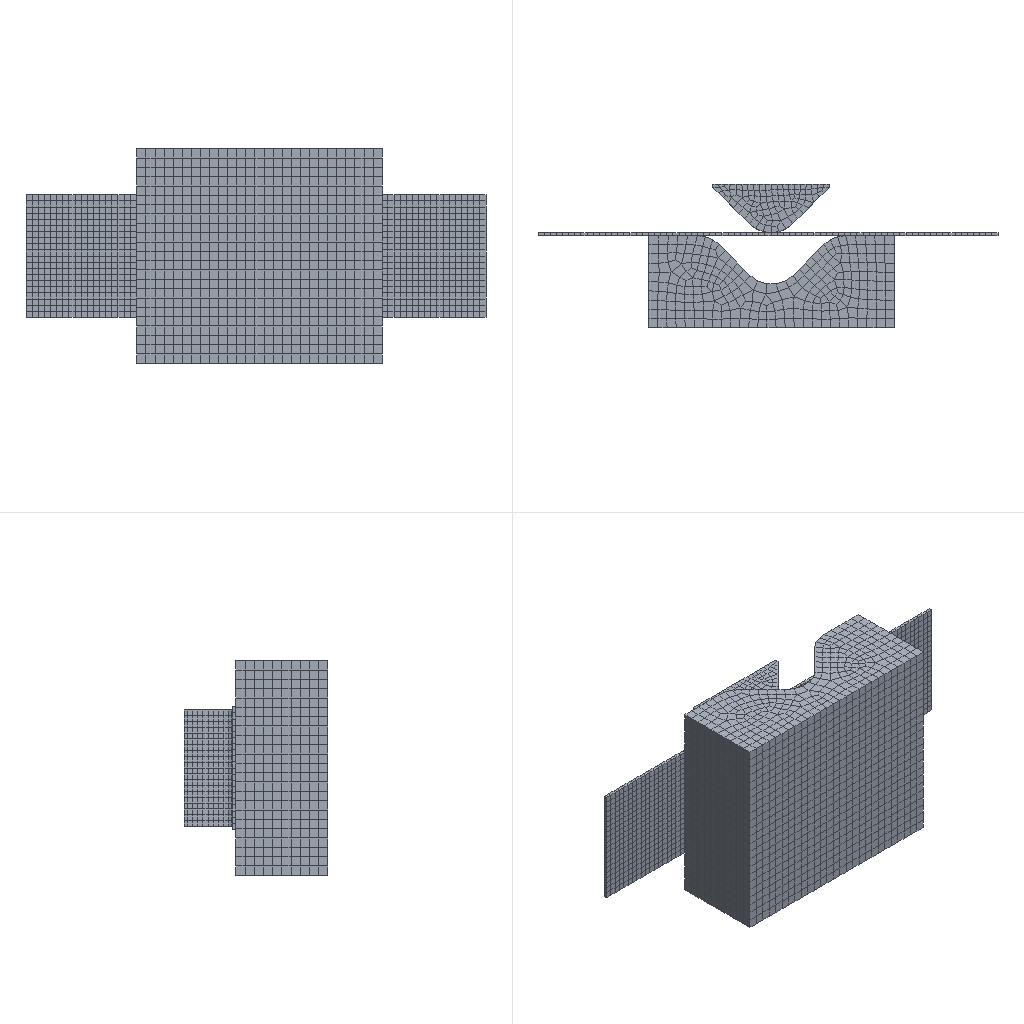Simulation study | abaqus
Set-up summary:
category,name,step,type,value,unit,region
solver,abaqus
solver,version,,,Abaqus/Standard 2020
units,not stated in the deck,,not stated
analysis,deck,,coupled temperature-displacement,coupled temperature-displacement
load_step,Step-1,Step-1,coupled temperature-displacement
load_step,Step-2,Step-2,coupled temperature-displacement
load_step,requested,,,2
mesh,nodes,,,12858
mesh,elements,,,9388
element_type,Q3D8R,,solid,9388
load,load commands in deck,,count,6
bc,support commands in deck,,count,21
material,BAN,,in results
material,MUJU,,in results
check,setup vs results,,match,"per instance, exact: element labels, types and connectivity; labels of the nodes the elements use; coordinates of those nodes at SINGLE_PRECISION in 3 of 3 instance(s)"
Abaqus input file, long lists of numbers shortened:
*Heading
** Job name: Job-1 Model name: Model-1
** Generated by: Abaqus/CAE 2020
*Preprint, echo=NO, model=NO, history=NO, contact=NO
**
** PARTS
**
*Part, name=work-1
*Node
      1,   160.87,   83.81,   69.627
      2,   158.87,   83.81,   69.627
** (3190 more lines like these left out)
*Element, type=Q3D8R
   1,  153,  154,  230,  229,    1,    2,   78,   77
   2,  154,  155,  231,  230,    2,    3,   79,   78
** (1498 more lines like these left out)
*Nset, nset=Set-1, generate
    1,  3192,     1
*Elset, elset=Set-1, generate
    1,  1500,     1
** Section: ban
*Solid Section, elset=Set-1, material=ban
,
*End Part
**
*Part, name=work-2
*Node
      1,   94.45,   95.668,    70.785
      2,   106.379,   107.597,    70.785
** (2560 more lines like these left out)
*Element, type=Q3D8R
   1,  117,  116,   86,  115,  239,  238,  208,  237
   2,   58,   69,   48,   45,  180,  191,  170,  167
** (1998 more lines like these left out)
*Nset, nset=Set-1, generate
    1,  2562,     1
*Elset, elset=Set-1, generate
    1,  2000,     1
** Section: muju
*Solid Section, elset=Set-1, material=muju
,
*End Part
**
*Part, name=work-3
*Node
      1,   111.165,   83.81,   124.661
      2,   127.022,   83.81,   124.661
** (7102 more lines like these left out)
*Element, type=Q3D8R
   1,  114,  185,   20,   21,  410,  481,  316,  317
   2,   85,   25,    5,   81,  381,  321,  301,  377
** (5886 more lines like these left out)
*Nset, nset=Set-1, generate
    1,  7104,     1
*Elset, elset=Set-1, generate
    1,  5888,     1
** Section: muju
*Solid Section, elset=Set-1, material=muju
,
*End Part
**
**
** ASSEMBLY
**
*Assembly, name=Assembly
**
*Instance, name=work-1-1, part=work-1
  -47.022,   -53.81,  -124.661
*End Instance
**
*Instance, name=work-2-1, part=work-2
  -47.531,   -61.739,   -124.819
*End Instance
**
*Instance, name=work-3-1, part=work-3
  -47.022,   -53.81,  -124.661
*End Instance
**
*Nset, nset=Set-1, instance=work-3-1
   16,   17,   44,   45,   46,   47,   48,   49,   50,   51,   52,   53,   54,   55,   56,   57
   58,   59,   60,   61,   62,   63,   64,   65,   66,   67,   68,   69,  312,  313,  340,  341
** (40 more lines like these left out)
*Elset, elset=Set-1, instance=work-3-1
    4,    5,    7,   20,   22,   34,   35,   36,   37,   39,   42,   43,   47,   49,   52,   57
   58,   61,   62,   77,   80,   82,   86,   88,   90,   98,  101,  260,  261,  263,  276,  278
** (37 more lines like these left out)
*Nset, nset=Set-2, instance=work-1-1, generate
    1,  3117,    76
*Elset, elset=Set-2, instance=work-1-1, generate
    1,  1426,    75
*Nset, nset=Set-3, instance=work-2-1
   10,   11,   24,   25,   26,   27,   28,   29,   30,   31,   32,   33,   34,   35,   36,   37
   38,   39,   40,   41,   42,  132,  133,  146,  147,  148,  149,  150,  151,  152,  153,  154
** (26 more lines like these left out)
*Elset, elset=Set-3, instance=work-2-1
    3,    5,    6,    7,   11,   15,   17,   18,   22,   24,   25,   26,   28,   32,   36,   41
   42,   47,   51,   78,  103,  105,  106,  107,  111,  115,  117,  118,  122,  124,  125,  126
** (23 more lines like these left out)
*Nset, nset=Set-4, instance=work-1-1, generate
    1,  3192,     1
*Nset, nset=Set-4, instance=work-2-1, generate
    1,  2562,     1
*Nset, nset=Set-4, instance=work-3-1, generate
    1,  7104,     1
*Elset, elset=Set-4, instance=work-1-1, generate
    1,  1500,     1
*Elset, elset=Set-4, instance=work-2-1, generate
    1,  2000,     1
*Elset, elset=Set-4, instance=work-3-1, generate
    1,  5888,     1
*Nset, nset=Set-5, instance=work-1-1
    1,   76,   77,  152,  153,  228,  229,  304,  305,  380,  381,  456,  457,  532,  533,  608
  609,  684,  685,  760,  761,  836,  837,  912,  913,  988,  989, 1064, 1065, 1140, 1141, 1216
** (4 more lines like these left out)
*Elset, elset=Set-5, instance=work-1-1
    1,   75,   76,  150,  151,  225,  226,  300,  301,  375,  376,  450,  451,  525,  526,  600
  601,  675,  676,  750,  751,  825,  826,  900,  901,  975,  976, 1050, 1051, 1125, 1126, 1200
** (1 more lines like these left out)
*Nset, nset=Set-6, instance=work-1-1
    1,   76,   77,  152,  153,  228,  229,  304,  305,  380,  381,  456,  457,  532,  533,  608
  609,  684,  685,  760,  761,  836,  837,  912,  913,  988,  989, 1064, 1065, 1140, 1141, 1216
** (4 more lines like these left out)
*Elset, elset=Set-6, instance=work-1-1
    1,   75,   76,  150,  151,  225,  226,  300,  301,  375,  376,  450,  451,  525,  526,  600
  601,  675,  676,  750,  751,  825,  826,  900,  901,  975,  976, 1050, 1051, 1125, 1126, 1200
** (1 more lines like these left out)
*Elset, elset=_Surf-1_S4, internal, instance=work-1-1, generate
   75,  1500,    75
*Surface, type=ELEMENT, name=Surf-1
_Surf-1_S4, S4
*Elset, elset=_Surf-6_S1, internal, instance=work-1-1, generate
 1426,  1500,     1
*Elset, elset=_Surf-6_S6, internal, instance=work-1-1, generate
    1,  1426,    75
*Elset, elset=_Surf-6_S2, internal, instance=work-1-1, generate
  1,  75,   1
*Elset, elset=_Surf-6_S4, internal, instance=work-1-1, generate
   75,  1500,    75
*Elset, elset=_Surf-6_S5, internal, instance=work-1-1, generate
    1,  1500,     1
*Elset, elset=_Surf-6_S3, internal, instance=work-1-1, generate
    1,  1500,     1
*Surface, type=ELEMENT, name=Surf-6
_Surf-6_S1, S1
_Surf-6_S6, S6
_Surf-6_S2, S2
_Surf-6_S4, S4
_Surf-6_S5, S5
_Surf-6_S3, S3
*Elset, elset=_Surf-7_S3, internal, instance=work-2-1
    3,    5,    6,   11,   15,   17,   24,   25,   28,   30,   32,   41,   42,   51,   76,   79
  103,  105,  106,  111,  115,  117,  124,  125,  128,  130,  132,  141,  142,  151,  176,  179
** (18 more lines like these left out)
*Elset, elset=_Surf-7_S3, internal, instance=work-3-1
   17,   23,   27,   36,   44,   59,   64,   69,   79,   81,  100,  104,  273,  279,  283,  292
  300,  315,  320,  325,  335,  337,  356,  360,  529,  535,  539,  548,  556,  571,  576,  581
** (16 more lines like these left out)
*Elset, elset=_Surf-7_S6, internal, instance=work-2-1
   10,   18,   31,   32,   33,   37,   46,   47,   52,   57,   60,   78,  110,  118,  131,  132
  133,  137,  146,  147,  152,  157,  160,  178,  210,  218,  231,  232,  233,  237,  246,  247
** (13 more lines like these left out)
*Elset, elset=_Surf-7_S6, internal, instance=work-3-1
    3,    9,   10,   11,   12,   20,   21,   30,   32,   35,   38,   43,   47,   49,   51,   52
   57,   58,   61,   62,   70,   87,  110,  113,  259,  265,  266,  267,  268,  276,  277,  286
** (33 more lines like these left out)
*Elset, elset=_Surf-7_S5, internal, instance=work-2-1
    7,   18,   19,   22,   26,   36,   40,   53,  107,  118,  119,  122,  126,  136,  140,  153
  207,  218,  219,  222,  226,  236,  240,  253,  307,  318,  319,  322,  326,  336,  340,  353
** (8 more lines like these left out)
*Elset, elset=_Surf-7_S5, internal, instance=work-3-1
    1,   15,   31,   39,   41,   62,   63,   68,   72,  102,  103,  107,  116,  120,  129,  257
  271,  287,  295,  297,  318,  319,  324,  328,  358,  359,  363,  372,  376,  385,  513,  527
** (20 more lines like these left out)
*Elset, elset=_Surf-7_S4, internal, instance=work-2-1
   39,   62,   65,   70,   74,   75,  139,  162,  165,  170,  174,  175,  239,  262,  265,  270
  274,  275,  339,  362,  365,  370,  374,  375,  439,  462,  465,  470,  474,  475,  539,  562
** (6 more lines like these left out)
*Elset, elset=_Surf-7_S4, internal, instance=work-3-1
    2,    4,    5,    7,   13,   22,   26,   29,   31,   34,   37,   39,   42,   54,   63,   73
   77,   80,   82,   85,   86,   88,   90,   98,  101,  109,  119,  258,  260,  261,  263,  269
** (37 more lines like these left out)
*Elset, elset=_Surf-7_S2, internal, instance=work-2-1, generate
 1901,  2000,     1
*Elset, elset=_Surf-7_S2, internal, instance=work-3-1, generate
 5633,  5888,     1
*Elset, elset=_Surf-7_S1, internal, instance=work-2-1, generate
   1,  100,    1
*Elset, elset=_Surf-7_S1, internal, instance=work-3-1, generate
   1,  256,    1
*Surface, type=ELEMENT, name=Surf-7
_Surf-7_S3, S3
_Surf-7_S6, S6
_Surf-7_S4, S4
_Surf-7_S2, S2
_Surf-7_S5, S5
_Surf-7_S1, S1
*Elset, elset=_Surf-8_S1, internal, instance=work-1-1, generate
 1426,  1500,     1
*Elset, elset=_Surf-8_S1, internal, instance=work-2-1, generate
   1,  100,    1
*Elset, elset=_Surf-8_S1, internal, instance=work-3-1, generate
   1,  256,    1
*Elset, elset=_Surf-8_S6, internal, instance=work-1-1, generate
    1,  1426,    75
*Elset, elset=_Surf-8_S6, internal, instance=work-2-1
   10,   18,   31,   32,   33,   37,   46,   47,   52,   57,   60,   78,  110,  118,  131,  132
  133,  137,  146,  147,  152,  157,  160,  178,  210,  218,  231,  232,  233,  237,  246,  247
** (13 more lines like these left out)
*Elset, elset=_Surf-8_S6, internal, instance=work-3-1
    3,    9,   10,   11,   12,   20,   21,   30,   32,   35,   38,   43,   47,   49,   51,   52
   57,   58,   61,   62,   70,   87,  110,  113,  259,  265,  266,  267,  268,  276,  277,  286
** (33 more lines like these left out)
*Elset, elset=_Surf-8_S2, internal, instance=work-1-1, generate
  1,  75,   1
*Elset, elset=_Surf-8_S2, internal, instance=work-2-1, generate
 1901,  2000,     1
*Elset, elset=_Surf-8_S2, internal, instance=work-3-1, generate
 5633,  5888,     1
*Elset, elset=_Surf-8_S4, internal, instance=work-1-1, generate
   75,  1500,    75
*Elset, elset=_Surf-8_S4, internal, instance=work-2-1
   39,   62,   65,   70,   74,   75,  139,  162,  165,  170,  174,  175,  239,  262,  265,  270
  274,  275,  339,  362,  365,  370,  374,  375,  439,  462,  465,  470,  474,  475,  539,  562
** (6 more lines like these left out)
*Elset, elset=_Surf-8_S4, internal, instance=work-3-1
    2,    4,    5,    7,   13,   22,   26,   29,   31,   34,   37,   39,   42,   54,   63,   73
   77,   80,   82,   85,   86,   88,   90,   98,  101,  109,  119,  258,  260,  261,  263,  269
** (37 more lines like these left out)
*Elset, elset=_Surf-8_S5, internal, instance=work-1-1, generate
    1,  1500,     1
*Elset, elset=_Surf-8_S5, internal, instance=work-2-1
    7,   18,   19,   22,   26,   36,   40,   53,  107,  118,  119,  122,  126,  136,  140,  153
  207,  218,  219,  222,  226,  236,  240,  253,  307,  318,  319,  322,  326,  336,  340,  353
** (8 more lines like these left out)
*Elset, elset=_Surf-8_S5, internal, instance=work-3-1
    1,   15,   31,   39,   41,   62,   63,   68,   72,  102,  103,  107,  116,  120,  129,  257
  271,  287,  295,  297,  318,  319,  324,  328,  358,  359,  363,  372,  376,  385,  513,  527
** (20 more lines like these left out)
*Elset, elset=_Surf-8_S3, internal, instance=work-1-1, generate
    1,  1500,     1
*Elset, elset=_Surf-8_S3, internal, instance=work-2-1
    3,    5,    6,   11,   15,   17,   24,   25,   28,   30,   32,   41,   42,   51,   76,   79
  103,  105,  106,  111,  115,  117,  124,  125,  128,  130,  132,  141,  142,  151,  176,  179
** (18 more lines like these left out)
*Elset, elset=_Surf-8_S3, internal, instance=work-3-1
   17,   23,   27,   36,   44,   59,   64,   69,   79,   81,  100,  104,  273,  279,  283,  292
  300,  315,  320,  325,  335,  337,  356,  360,  529,  535,  539,  548,  556,  571,  576,  581
** (16 more lines like these left out)
*Surface, type=ELEMENT, name=Surf-8
_Surf-8_S1, S1
_Surf-8_S6, S6
_Surf-8_S2, S2
_Surf-8_S4, S4
_Surf-8_S5, S5
_Surf-8_S3, S3
*Elset, elset=_m_Surf-2_S3, internal, instance=work-2-1
   30,   76,   79,  130,  176,  179,  230,  276,  279,  330,  376,  379,  430,  476,  479,  530
  576,  579,  630,  676,  679,  730,  776,  779,  830,  876,  879,  930,  976,  979, 1030, 1076
** (2 more lines like these left out)
*Elset, elset=_m_Surf-2_S6, internal, instance=work-2-1
   10,   31,   33,   37,   46,   52,   57,   60,  110,  131,  133,  137,  146,  152,  157,  160
  210,  231,  233,  237,  246,  252,  257,  260,  310,  331,  333,  337,  346,  352,  357,  360
** (8 more lines like these left out)
*Elset, elset=_m_Surf-2_S5, internal, instance=work-2-1
   19,   40,   53,  119,  140,  153,  219,  240,  253,  319,  340,  353,  419,  440,  453,  519
  540,  553,  619,  640,  653,  719,  740,  753,  819,  840,  853,  919,  940,  953, 1019, 1040
** (2 more lines like these left out)
*Elset, elset=_m_Surf-2_S4, internal, instance=work-2-1
   39,   62,   65,   70,   74,   75,  139,  162,  165,  170,  174,  175,  239,  262,  265,  270
  274,  275,  339,  362,  365,  370,  374,  375,  439,  462,  465,  470,  474,  475,  539,  562
** (6 more lines like these left out)
*Surface, type=ELEMENT, name=m_Surf-2
_m_Surf-2_S3, S3
_m_Surf-2_S6, S6
_m_Surf-2_S4, S4
_m_Surf-2_S5, S5
*Elset, elset=_m_Surf-4_S3, internal, instance=work-3-1
   23,   27,   44,   59,   69,   79,   81,  104,  279,  283,  300,  315,  325,  335,  337,  360
  535,  539,  556,  571,  581,  591,  593,  616,  791,  795,  812,  827,  837,  847,  849,  872
** (10 more lines like these left out)
*Elset, elset=_m_Surf-4_S5, internal, instance=work-3-1
    1,   15,   31,   41,   72,  120,  129,  257,  271,  287,  297,  328,  376,  385,  513,  527
  543,  553,  584,  632,  641,  769,  783,  799,  809,  840,  888,  897, 1025, 1039, 1055, 1065
** (9 more lines like these left out)
*Elset, elset=_m_Surf-4_S4, internal, instance=work-3-1
    2,   13,   26,   54,   63,   73,  119,  258,  269,  282,  310,  319,  329,  375,  514,  525
  538,  566,  575,  585,  631,  770,  781,  794,  822,  831,  841,  887, 1026, 1037, 1050, 1078
** (9 more lines like these left out)
*Elset, elset=_m_Surf-4_S6, internal, instance=work-3-1
    3,   10,   11,   12,   21,   30,   51,   70,  113,  259,  266,  267,  268,  277,  286,  307
  326,  369,  515,  522,  523,  524,  533,  542,  563,  582,  625,  771,  778,  779,  780,  789
** (11 more lines like these left out)
*Surface, type=ELEMENT, name=m_Surf-4
_m_Surf-4_S3, S3
_m_Surf-4_S5, S5
_m_Surf-4_S4, S4
_m_Surf-4_S6, S6
*Elset, elset=_s_Surf-2_S5, internal, instance=work-1-1, generate
    1,  1500,     1
*Surface, type=ELEMENT, name=s_Surf-2
_s_Surf-2_S5, S5
*Elset, elset=_s_Surf-4_S3, internal, instance=work-1-1, generate
    1,  1500,     1
*Surface, type=ELEMENT, name=s_Surf-4
_s_Surf-4_S3, S3
*End Assembly
*Amplitude, name=Amp-1, definition=PERIODIC
1,         125600.,              0.,              2.
          0.008,              0.
**
** MATERIALS
**
*Material, name=ban
*Conductivity
175., 20.
185.,100.
193.,200.
193.,300.
190.,400.
188.,500.
*Density
 2.7e-09,
*Elastic
82000., 0.33,  20.
75000., 0.33, 100.
69000., 0.33, 200.
60000., 0.33, 300.
*Electrical Conductivity
 0.02665,
*Expansion
 2.23e-05, 25.
 2.28e-05,100.
 2.47e-05,200.
 2.55e-05,300.
 2.67e-05,400.
  2.7e-05,500.
*Specific Heat
  8.5e+08, 25.
    9e+08,100.
  9.5e+08,200.
  9.7e+08,300.
    1e+09,400.
 1.08e+09,500.
*Material, name=muju
*Conductivity
  40., 25.
 39.5,100.
 38.8,200.
 38.2,300.
 37.6,400.
  37.,500.
*Density
 7.8e-09,
*Elastic
210000., 0.3
*Electrical Conductivity
 2e-07,
*Specific Heat
 4.65e+08,
**
** INTERACTION PROPERTIES
**
*Surface Interaction, name=IntProp-1
1.,
*Friction, slip tolerance=0.005
 0.2,
*Surface Behavior, pressure-overclosure=HARD
*Gap Conductance
 0.5,    0.
  0., 0.001
**
** PHYSICAL CONSTANTS
**
*Physical Constants, absolute zero=-273., stefan boltzmann=5.67e-08
**
** PREDEFINED FIELDS
**
** Name: Predefined Field-1   Type: Temperature
*Initial Conditions, type=TEMPERATURE
Set-4, 20.
**
** INTERACTIONS
**
** Interaction: Int-1
*Contact Pair, interaction=IntProp-1, type=SURFACE TO SURFACE
m_Surf-2, s_Surf-2
** Interaction: Int-2
*Contact Pair, interaction=IntProp-1, type=SURFACE TO SURFACE
s_Surf-4, m_Surf-4
** ----------------------------------------------------------------
**
** STEP: Step-1
**
*Step, name=Step-1, nlgeom=YES, inc=1000
*Coupled Temperature-displacement, electrical, creep=none, deltmx=1e+10, stabilize=0.0002, allsdtol=0.05, continue=NO
0.01, 3.4, 1e-05, 3.4
**
** BOUNDARY CONDITIONS
**
** Name: BC-2 Type: 电势
*Boundary
Set-2, 9, 9
** Name: BC-5 Type: 位移/转角
*Boundary
Set-6, 2, 2
** Name: [REDACTED] : Symmetric / antisymmetric / fully fixed
*Boundary
Set-1, ENCASTRE
** Name: [REDACTED] : Speed/Angular velocity
*Boundary, amplitude=Amp-1, type=VELOCITY
Set-3, 1, 1
Set-3, 2, 2, -2.
Set-3, 3, 3
Set-3, 4, 4
Set-3, 5, 5
Set-3, 6, 6
**
** LOADS
**
** Name: Load-1   Type: Surface current
*Dsecurrent
Surf-1,CS,3.2
**
** INTERACTIONS
**
** Interaction: Int-3
*Sfilm
Surf-6, F, 20., 0.001
** Interaction: Int-4
*Sfilm
Surf-7, F, 20., 0.001
** Interaction: Int-5
*Sradiate
Surf-8, R, 20., 0.3
**
** OUTPUT REQUESTS
**
*Restart, write, frequency=0
**
** FIELD OUTPUT: F-Output-1
**
*Output, field
*Node Output
CECHG, CECUR, CF, EPOT, NT, RCHG, RECUR, RF
RFL, RM, RT, U
*Element Output, directions=YES
E, ECD, EFLX, EPG, HFL, LE, MISES, MISESMAX, MISESONLY, NCURS, PE, PEEQ, PEEQMAX, PEEQT, PEMAG, S
SF, SSAVG, TEMP, VEEQ, YIELDPOT
*Contact Output
CDISP, CSTRESS, ECD, ECDA, ECDT, ECDTA
**
** HISTORY OUTPUT: H-Output-1
**
*Output, history, variable=PRESELECT
*End Step
** ----------------------------------------------------------------
**
** STEP: Step-2
**
*Step, name=Step-2, nlgeom=YES, inc=1000
*Coupled Temperature-displacement, electrical, creep=none, deltmx=1e+06, stabilize=0.0002, allsdtol=0.05, continue=NO
0.01, 2., 2e-05, 2.
**
** BOUNDARY CONDITIONS
**
** Name: BC-2 Type: 电势
*Boundary, op=NEW
Set-2, 9, 9
** Name: BC-5 Type: 位移/转角
*Boundary, op=NEW
Set-6, 2, 2
** Name: [REDACTED] : Symmetric / antisymmetric / fully fixed
*Boundary, op=NEW
Set-1, ENCASTRE
** Name: [REDACTED] : Speed/Angular velocity
*Boundary, op=NEW, type=VELOCITY
Set-3, 1, 1
Set-3, 2, 2, 10.
Set-3, 3, 3
Set-3, 4, 4
Set-3, 5, 5
Set-3, 6, 6
**
** OUTPUT REQUESTS
**
*Restart, write, frequency=0
**
** FIELD OUTPUT: F-Output-1
**
*Output, field
*Node Output
CECHG, CECUR, CF, EPOT, NT, RCHG, RECUR, RF
RFL, RM, RT, U
*Element Output, directions=YES
E, ECD, EFLX, EPG, HFL, LE, MISES, MISESMAX, MISESONLY, NCURS, PE, PEEQ, PEEQMAX, PEEQT, PEMAG, S
SF, SSAVG, TEMP, VEEQ, YIELDPOT
*Contact Output
CDISP, CSTRESS, ECD, ECDA, ECDT, ECDTA
**
** HISTORY OUTPUT: H-Output-1
**
*Output, history, variable=PRESELECT
*End Step
Results summary:
result,step,,partial,increments=39 time=3.4/3.4
result,step,,completed,increments=48 time=2.0/2.0
result,analysis,,,"coupled temperature-displacement, steady state"
result,last_loadstep,,,2
result,primary field,,,"U, NT11"
result,reaction total,,FX,-0.0,model units
result,reaction total,,FY,4e-06,model units
result,reaction total,,FZ,0.0,model units